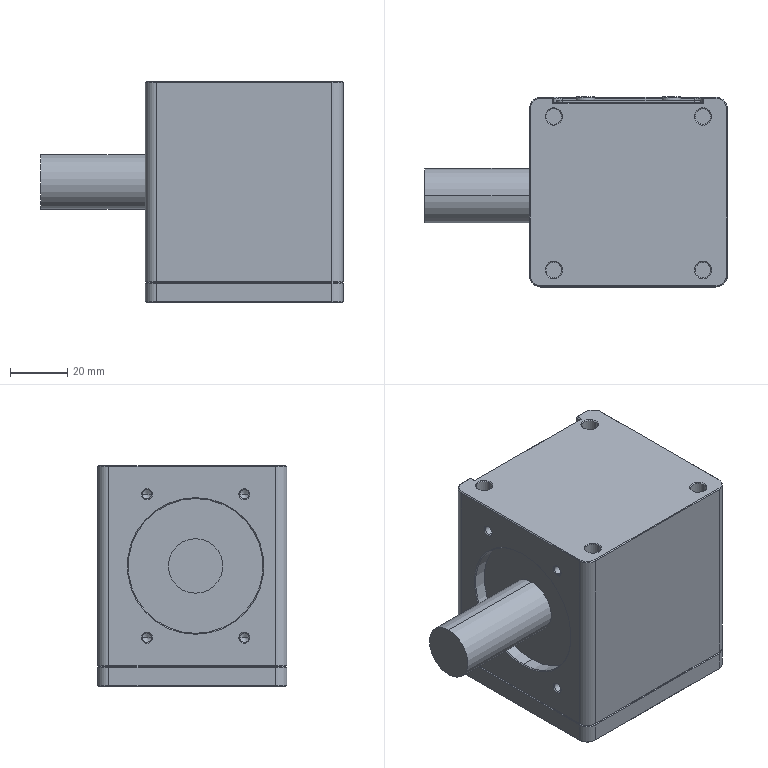Part | SolidWorks | features BaseBody 2 | 2 solids | 287 faces | box 105.5 x 66.1 x 77 mm | volume 335496 mm3 | plane 109 | cone 86 | cylinder 80 | spline 12 | commonest cylinder face diameters 3.3 x16 5.5 x16 3.4 x8 6.5 x8 8 x8 10 x8